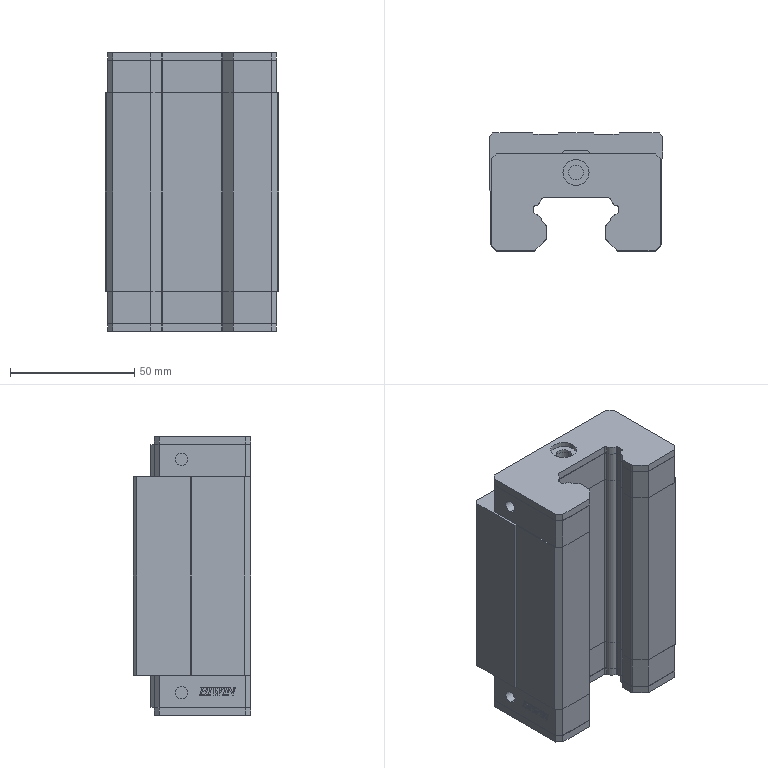Part | STEP file | HGH35C | 5 solids | 598 faces | box 70 x 47.5 x 112.4 mm | volume 276753 mm3 | plane 428 | cylinder 138 | cone 32 | commonest cylinder face diameters 0.25 x34 2.4 x20 6.5 x20 0.125 x18 5 x8 6 x8